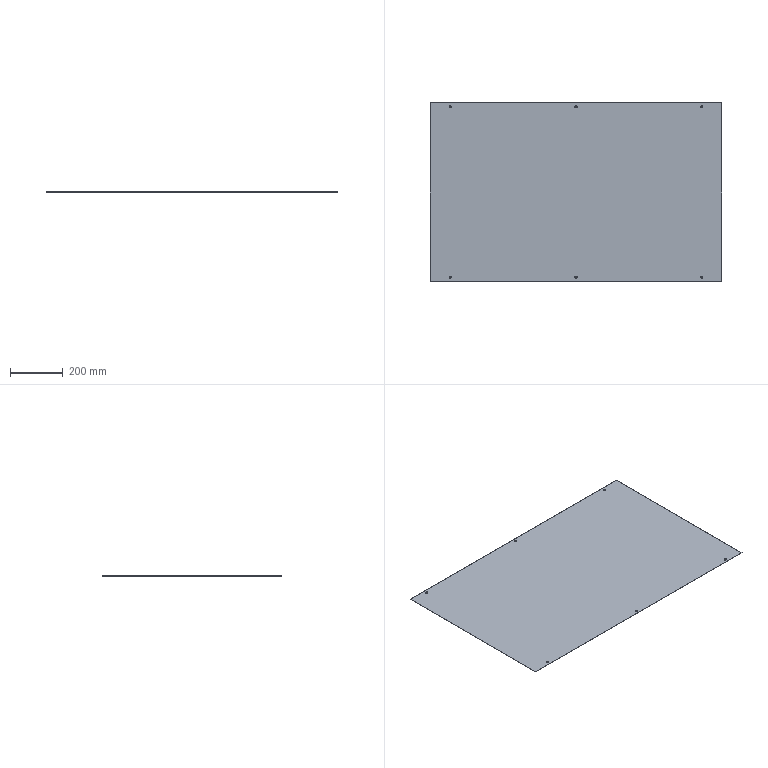Part | SolidWorks | features Cut 1, Extrusion 1 | 1 solid | 18 faces | box 1100 x 672 x 0.8 mm | volume 591119 mm3 | cylinder 12 | plane 6 | commonest cylinder face diameters 8 x12
STEP:
#1=CARTESIAN_POINT('',(-471.,321.,0.8));
#2=VERTEX_POINT('',#1);
#3=CARTESIAN_POINT('',(-479.,321.,0.8));
#4=VERTEX_POINT('',#3);
#5=CARTESIAN_POINT('',(-475.,321.,0.8));
#6=DIRECTION('',(0.,0.,-1.));
#7=DIRECTION('',(-1.,0.,0.));
#8=AXIS2_PLACEMENT_3D('',#5,#6,#7);
#9=CIRCLE('',#8,4.);
#10=EDGE_CURVE('',#2,#4,#9,.T.);
#11=ORIENTED_EDGE('',*,*,#10,.F.);
#12=CARTESIAN_POINT('',(-471.,321.,0.));
#13=VERTEX_POINT('',#12);
#14=CARTESIAN_POINT('',(-471.,321.,0.8));
#15=DIRECTION('',(0.,0.,-1.));
#16=VECTOR('',#15,1000.);
#17=LINE('',#14,#16);
#18=EDGE_CURVE('',#2,#13,#17,.T.);
#19=ORIENTED_EDGE('',*,*,#18,.T.);
#20=CARTESIAN_POINT('',(-479.,321.,0.));
#21=VERTEX_POINT('',#20);
#22=CARTESIAN_POINT('',(-475.,321.,0.));
#23=DIRECTION('',(0.,0.,-1.));
#24=DIRECTION('',(-1.,0.,0.));
#25=AXIS2_PLACEMENT_3D('',#22,#23,#24);
#26=CIRCLE('',#25,4.);
#27=EDGE_CURVE('',#13,#21,#26,.T.);
#28=ORIENTED_EDGE('',*,*,#27,.T.);
#29=CARTESIAN_POINT('',(-479.,321.,0.8));
#30=DIRECTION('',(0.,0.,-1.));
#31=VECTOR('',#30,1000.);
#32=LINE('',#29,#31);
#33=EDGE_CURVE('',#4,#21,#32,.T.);
#34=ORIENTED_EDGE('',*,*,#33,.F.);
#35=EDGE_LOOP('',(#11,#19,#28,#34));
#36=FACE_OUTER_BOUND('',#35,.T.);
#37=CARTESIAN_POINT('',(-475.,321.,0.8));
#38=DIRECTION('',(0.,0.,-1.));
#39=DIRECTION('',(-1.,0.,0.));
#40=AXIS2_PLACEMENT_3D('',#37,#38,#39);
#41=CYLINDRICAL_SURFACE('',#40,4.);
#42=ADVANCED_FACE('',(#36),#41,.F.);
#43=CARTESIAN_POINT('',(479.,321.,0.8));
#44=VERTEX_POINT('',#43);
#45=CARTESIAN_POINT('',(471.,321.,0.8));
#46=VERTEX_POINT('',#45);
#47=CARTESIAN_POINT('',(475.,321.,0.8));
#48=DIRECTION('',(0.,0.,-1.));
#49=DIRECTION('',(1.,0.,0.));
#50=AXIS2_PLACEMENT_3D('',#47,#48,#49);
#51=CIRCLE('',#50,4.);
#52=EDGE_CURVE('',#44,#46,#51,.T.);
#53=ORIENTED_EDGE('',*,*,#52,.F.);
#54=CARTESIAN_POINT('',(479.,321.,0.));
#55=VERTEX_POINT('',#54);
#56=CARTESIAN_POINT('',(479.,321.,0.8));
#57=DIRECTION('',(0.,0.,-1.));
#58=VECTOR('',#57,1000.);
#59=LINE('',#56,#58);
#60=EDGE_CURVE('',#44,#55,#59,.T.);
#61=ORIENTED_EDGE('',*,*,#60,.T.);
#62=CARTESIAN_POINT('',(471.,321.,0.));
#63=VERTEX_POINT('',#62);
#64=CARTESIAN_POINT('',(475.,321.,0.));
#65=DIRECTION('',(0.,0.,-1.));
#66=DIRECTION('',(1.,0.,0.));
#67=AXIS2_PLACEMENT_3D('',#64,#65,#66);
#68=CIRCLE('',#67,4.);
#69=EDGE_CURVE('',#55,#63,#68,.T.);
#70=ORIENTED_EDGE('',*,*,#69,.T.);
#71=CARTESIAN_POINT('',(471.,321.,0.8));
#72=DIRECTION('',(0.,0.,-1.));
#73=VECTOR('',#72,1000.);
#74=LINE('',#71,#73);
#75=EDGE_CURVE('',#46,#63,#74,.T.);
#76=ORIENTED_EDGE('',*,*,#75,.F.);
#77=EDGE_LOOP('',(#53,#61,#70,#76));
#78=FACE_OUTER_BOUND('',#77,.T.);
#79=CARTESIAN_POINT('',(475.,321.,0.8));
#80=DIRECTION('',(0.,0.,-1.));
#81=DIRECTION('',(-1.,0.,0.));
#82=AXIS2_PLACEMENT_3D('',#79,#80,#81);
#83=CYLINDRICAL_SURFACE('',#82,4.);
#84=ADVANCED_FACE('',(#78),#83,.F.);
#85=CARTESIAN_POINT('',(479.,-321.,0.8));
#86=VERTEX_POINT('',#85);
#87=CARTESIAN_POINT('',(471.,-321.,0.8));
#88=VERTEX_POINT('',#87);
#89=CARTESIAN_POINT('',(475.,-321.,0.8));
#90=DIRECTION('',(0.,0.,-1.));
#91=DIRECTION('',(-1.,0.,0.));
#92=AXIS2_PLACEMENT_3D('',#89,#90,#91);
#93=CIRCLE('',#92,4.);
#94=EDGE_CURVE('',#86,#88,#93,.T.);
#95=ORIENTED_EDGE('',*,*,#94,.F.);
#96=CARTESIAN_POINT('',(479.,-321.,0.));
#97=VERTEX_POINT('',#96);
#98=CARTESIAN_POINT('',(479.,-321.,0.8));
#99=DIRECTION('',(0.,0.,-1.));
#100=VECTOR('',#99,1000.);
#101=LINE('',#98,#100);
#102=EDGE_CURVE('',#86,#97,#101,.T.);
#103=ORIENTED_EDGE('',*,*,#102,.T.);
#104=CARTESIAN_POINT('',(471.,-321.,0.));
#105=VERTEX_POINT('',#104);
#106=CARTESIAN_POINT('',(475.,-321.,0.));
#107=DIRECTION('',(0.,0.,-1.));
#108=DIRECTION('',(-1.,0.,0.));
#109=AXIS2_PLACEMENT_3D('',#106,#107,#108);
#110=CIRCLE('',#109,4.);
#111=EDGE_CURVE('',#97,#105,#110,.T.);
#112=ORIENTED_EDGE('',*,*,#111,.T.);
#113=CARTESIAN_POINT('',(471.,-321.,0.8));
#114=DIRECTION('',(0.,0.,-1.));
#115=VECTOR('',#114,1000.);
#116=LINE('',#113,#115);
#117=EDGE_CURVE('',#88,#105,#116,.T.);
#118=ORIENTED_EDGE('',*,*,#117,.F.);
#119=EDGE_LOOP('',(#95,#103,#112,#118));
#120=FACE_OUTER_BOUND('',#119,.T.);
#121=CARTESIAN_POINT('',(475.,-321.,0.8));
#122=DIRECTION('',(0.,0.,-1.));
#123=DIRECTION('',(-1.,0.,0.));
#124=AXIS2_PLACEMENT_3D('',#121,#122,#123);
#125=CYLINDRICAL_SURFACE('',#124,4.);
#126=ADVANCED_FACE('',(#120),#125,.F.);
#127=CARTESIAN_POINT('',(-471.,-321.,0.8));
#128=VERTEX_POINT('',#127);
#129=CARTESIAN_POINT('',(-479.,-321.,0.8));
#130=VERTEX_POINT('',#129);
#131=CARTESIAN_POINT('',(-475.,-321.,0.8));
#132=DIRECTION('',(0.,0.,-1.));
#133=DIRECTION('',(1.,0.,0.));
#134=AXIS2_PLACEMENT_3D('',#131,#132,#133);
#135=CIRCLE('',#134,4.);
#136=EDGE_CURVE('',#128,#130,#135,.T.);
#137=ORIENTED_EDGE('',*,*,#136,.F.);
#138=CARTESIAN_POINT('',(-471.,-321.,0.));
#139=VERTEX_POINT('',#138);
#140=CARTESIAN_POINT('',(-471.,-321.,0.8));
#141=DIRECTION('',(0.,0.,-1.));
#142=VECTOR('',#141,1000.);
#143=LINE('',#140,#142);
#144=EDGE_CURVE('',#128,#139,#143,.T.);
#145=ORIENTED_EDGE('',*,*,#144,.T.);
#146=CARTESIAN_POINT('',(-479.,-321.,0.));
#147=VERTEX_POINT('',#146);
#148=CARTESIAN_POINT('',(-475.,-321.,0.));
#149=DIRECTION('',(0.,0.,-1.));
#150=DIRECTION('',(1.,0.,0.));
#151=AXIS2_PLACEMENT_3D('',#148,#149,#150);
#152=CIRCLE('',#151,4.);
#153=EDGE_CURVE('',#139,#147,#152,.T.);
#154=ORIENTED_EDGE('',*,*,#153,.T.);
#155=CARTESIAN_POINT('',(-479.,-321.,0.8));
#156=DIRECTION('',(0.,0.,-1.));
#157=VECTOR('',#156,1000.);
#158=LINE('',#155,#157);
#159=EDGE_CURVE('',#130,#147,#158,.T.);
#160=ORIENTED_EDGE('',*,*,#159,.F.);
#161=EDGE_LOOP('',(#137,#145,#154,#160));
#162=FACE_OUTER_BOUND('',#161,.T.);
#163=CARTESIAN_POINT('',(-475.,-321.,0.8));
#164=DIRECTION('',(0.,0.,-1.));
#165=DIRECTION('',(-1.,0.,0.));
#166=AXIS2_PLACEMENT_3D('',#163,#164,#165);
#167=CYLINDRICAL_SURFACE('',#166,4.);
#168=ADVANCED_FACE('',(#162),#167,.F.);
#169=CARTESIAN_POINT('',(4.,-321.,0.8));
#170=VERTEX_POINT('',#169);
#171=CARTESIAN_POINT('',(-4.,-321.,0.8));
#172=VERTEX_POINT('',#171);
#173=CARTESIAN_POINT('',(0.,-321.,0.8));
#174=DIRECTION('',(0.,0.,-1.));
#175=DIRECTION('',(1.,0.,0.));
#176=AXIS2_PLACEMENT_3D('',#173,#174,#175);
#177=CIRCLE('',#176,4.);
#178=EDGE_CURVE('',#170,#172,#177,.T.);
#179=ORIENTED_EDGE('',*,*,#178,.F.);
#180=CARTESIAN_POINT('',(4.,-321.,0.));
#181=VERTEX_POINT('',#180);
#182=CARTESIAN_POINT('',(4.,-321.,0.8));
#183=DIRECTION('',(0.,0.,-1.));
#184=VECTOR('',#183,1000.);
#185=LINE('',#182,#184);
#186=EDGE_CURVE('',#170,#181,#185,.T.);
#187=ORIENTED_EDGE('',*,*,#186,.T.);
#188=CARTESIAN_POINT('',(-4.,-321.,0.));
#189=VERTEX_POINT('',#188);
#190=CARTESIAN_POINT('',(0.,-321.,0.));
#191=DIRECTION('',(0.,0.,-1.));
#192=DIRECTION('',(1.,0.,0.));
#193=AXIS2_PLACEMENT_3D('',#190,#191,#192);
#194=CIRCLE('',#193,4.);
#195=EDGE_CURVE('',#181,#189,#194,.T.);
#196=ORIENTED_EDGE('',*,*,#195,.T.);
#197=CARTESIAN_POINT('',(-4.,-321.,0.8));
#198=DIRECTION('',(0.,0.,-1.));
#199=VECTOR('',#198,1000.);
#200=LINE('',#197,#199);
#201=EDGE_CURVE('',#172,#189,#200,.T.);
#202=ORIENTED_EDGE('',*,*,#201,.F.);
#203=EDGE_LOOP('',(#179,#187,#196,#202));
#204=FACE_OUTER_BOUND('',#203,.T.);
#205=CARTESIAN_POINT('',(0.,-321.,0.8));
#206=DIRECTION('',(0.,0.,-1.));
#207=DIRECTION('',(-1.,0.,0.));
#208=AXIS2_PLACEMENT_3D('',#205,#206,#207);
#209=CYLINDRICAL_SURFACE('',#208,4.);
#210=ADVANCED_FACE('',(#204),#209,.F.);
#211=CARTESIAN_POINT('',(4.,321.,0.8));
#212=VERTEX_POINT('',#211);
#213=CARTESIAN_POINT('',(-4.,321.,0.8));
#214=VERTEX_POINT('',#213);
#215=CARTESIAN_POINT('',(0.,321.,0.8));
#216=DIRECTION('',(0.,0.,-1.));
#217=DIRECTION('',(-1.,0.,0.));
#218=AXIS2_PLACEMENT_3D('',#215,#216,#217);
#219=CIRCLE('',#218,4.);
#220=EDGE_CURVE('',#212,#214,#219,.T.);
#221=ORIENTED_EDGE('',*,*,#220,.F.);
#222=CARTESIAN_POINT('',(4.,321.,0.));
#223=VERTEX_POINT('',#222);
#224=CARTESIAN_POINT('',(4.,321.,0.8));
#225=DIRECTION('',(0.,0.,-1.));
#226=VECTOR('',#225,1000.);
#227=LINE('',#224,#226);
#228=EDGE_CURVE('',#212,#223,#227,.T.);
#229=ORIENTED_EDGE('',*,*,#228,.T.);
#230=CARTESIAN_POINT('',(-4.,321.,0.));
#231=VERTEX_POINT('',#230);
#232=CARTESIAN_POINT('',(0.,321.,0.));
#233=DIRECTION('',(0.,0.,-1.));
#234=DIRECTION('',(-1.,0.,0.));
#235=AXIS2_PLACEMENT_3D('',#232,#233,#234);
#236=CIRCLE('',#235,4.);
#237=EDGE_CURVE('',#223,#231,#236,.T.);
#238=ORIENTED_EDGE('',*,*,#237,.T.);
#239=CARTESIAN_POINT('',(-4.,321.,0.8));
#240=DIRECTION('',(0.,0.,-1.));
#241=VECTOR('',#240,1000.);
#242=LINE('',#239,#241);
#243=EDGE_CURVE('',#214,#231,#242,.T.);
#244=ORIENTED_EDGE('',*,*,#243,.F.);
#245=EDGE_LOOP('',(#221,#229,#238,#244));
#246=FACE_OUTER_BOUND('',#245,.T.);
#247=CARTESIAN_POINT('',(0.,321.,0.8));
#248=DIRECTION('',(0.,0.,-1.));
#249=DIRECTION('',(-1.,0.,0.));
#250=AXIS2_PLACEMENT_3D('',#247,#248,#249);
#251=CYLINDRICAL_SURFACE('',#250,4.);
#252=ADVANCED_FACE('',(#246),#251,.F.);
#253=CARTESIAN_POINT('',(550.,-336.,0.));
#254=VERTEX_POINT('',#253);
#255=CARTESIAN_POINT('',(550.,336.,0.));
#256=VERTEX_POINT('',#255);
#257=CARTESIAN_POINT('',(550.,336.,0.));
#258=DIRECTION('',(0.,1.,0.));
#259=VECTOR('',#258,1000.);
#260=LINE('',#257,#259);
#261=EDGE_CURVE('',#254,#256,#260,.T.);
#262=ORIENTED_EDGE('',*,*,#261,.T.);
#263=CARTESIAN_POINT('',(550.,336.,0.8));
#264=VERTEX_POINT('',#263);
#265=CARTESIAN_POINT('',(550.,336.,0.8));
#266=DIRECTION('',(0.,0.,-1.));
#267=VECTOR('',#266,1000.);
#268=LINE('',#265,#267);
#269=EDGE_CURVE('',#264,#256,#268,.T.);
#270=ORIENTED_EDGE('',*,*,#269,.F.);
#271=CARTESIAN_POINT('',(550.,-336.,0.8));
#272=VERTEX_POINT('',#271);
#273=CARTESIAN_POINT('',(550.,336.,0.8));
#274=DIRECTION('',(0.,1.,0.));
#275=VECTOR('',#274,1000.);
#276=LINE('',#273,#275);
#277=EDGE_CURVE('',#272,#264,#276,.T.);
#278=ORIENTED_EDGE('',*,*,#277,.F.);
#279=CARTESIAN_POINT('',(550.,-336.,0.8));
#280=DIRECTION('',(0.,0.,-1.));
#281=VECTOR('',#280,1000.);
#282=LINE('',#279,#281);
#283=EDGE_CURVE('',#272,#254,#282,.T.);
#284=ORIENTED_EDGE('',*,*,#283,.T.);
#285=EDGE_LOOP('',(#262,#270,#278,#284));
#286=FACE_OUTER_BOUND('',#285,.T.);
#287=CARTESIAN_POINT('',(550.,336.,0.8));
#288=DIRECTION('',(-1.,0.,0.));
#289=DIRECTION('',(0.,-1.,0.));
#290=AXIS2_PLACEMENT_3D('',#287,#288,#289);
#291=PLANE('',#290);
#292=ADVANCED_FACE('',(#286),#291,.F.);
#293=CARTESIAN_POINT('',(-550.,336.,0.));
#294=VERTEX_POINT('',#293);
#295=CARTESIAN_POINT('',(-550.,336.,0.));
#296=DIRECTION('',(-1.,0.,0.));
#297=VECTOR('',#296,1000.);
#298=LINE('',#295,#297);
#299=EDGE_CURVE('',#256,#294,#298,.T.);
#300=ORIENTED_EDGE('',*,*,#299,.T.);
#301=CARTESIAN_POINT('',(-550.,336.,0.8));
#302=VERTEX_POINT('',#301);
#303=CARTESIAN_POINT('',(-550.,336.,0.8));
#304=DIRECTION('',(0.,0.,-1.));
#305=VECTOR('',#304,1000.);
#306=LINE('',#303,#305);
#307=EDGE_CURVE('',#302,#294,#306,.T.);
#308=ORIENTED_EDGE('',*,*,#307,.F.);
#309=CARTESIAN_POINT('',(-550.,336.,0.8));
#310=DIRECTION('',(-1.,0.,0.));
#311=VECTOR('',#310,1000.);
#312=LINE('',#309,#311);
#313=EDGE_CURVE('',#264,#302,#312,.T.);
#314=ORIENTED_EDGE('',*,*,#313,.F.);
#315=ORIENTED_EDGE('',*,*,#269,.T.);
#316=EDGE_LOOP('',(#300,#308,#314,#315));
#317=FACE_OUTER_BOUND('',#316,.T.);
#318=CARTESIAN_POINT('',(-550.,336.,0.8));
#319=DIRECTION('',(0.,-1.,0.));
#320=DIRECTION('',(0.,0.,-1.));
#321=AXIS2_PLACEMENT_3D('',#318,#319,#320);
#322=PLANE('',#321);
#323=ADVANCED_FACE('',(#317),#322,.F.);
#324=CARTESIAN_POINT('',(-550.,-336.,0.));
#325=VERTEX_POINT('',#324);
#326=CARTESIAN_POINT('',(-550.,336.,0.));
#327=DIRECTION('',(0.,-1.,0.));
#328=VECTOR('',#327,1000.);
#329=LINE('',#326,#328);
#330=EDGE_CURVE('',#294,#325,#329,.T.);
#331=ORIENTED_EDGE('',*,*,#330,.T.);
#332=CARTESIAN_POINT('',(-550.,-336.,0.8));
#333=VERTEX_POINT('',#332);
#334=CARTESIAN_POINT('',(-550.,-336.,0.8));
#335=DIRECTION('',(0.,0.,-1.));
#336=VECTOR('',#335,1000.);
#337=LINE('',#334,#336);
#338=EDGE_CURVE('',#333,#325,#337,.T.);
#339=ORIENTED_EDGE('',*,*,#338,.F.);
#340=CARTESIAN_POINT('',(-550.,336.,0.8));
#341=DIRECTION('',(0.,-1.,0.));
#342=VECTOR('',#341,1000.);
#343=LINE('',#340,#342);
#344=EDGE_CURVE('',#302,#333,#343,.T.);
#345=ORIENTED_EDGE('',*,*,#344,.F.);
#346=ORIENTED_EDGE('',*,*,#307,.T.);
#347=EDGE_LOOP('',(#331,#339,#345,#346));
#348=FACE_OUTER_BOUND('',#347,.T.);
#349=CARTESIAN_POINT('',(-550.,336.,0.8));
#350=DIRECTION('',(1.,0.,0.));
#351=DIRECTION('',(0.,1.,0.));
#352=AXIS2_PLACEMENT_3D('',#349,#350,#351);
#353=PLANE('',#352);
#354=ADVANCED_FACE('',(#348),#353,.F.);
#355=CARTESIAN_POINT('',(-550.,-336.,0.));
#356=DIRECTION('',(1.,0.,0.));
#357=VECTOR('',#356,1000.);
#358=LINE('',#355,#357);
#359=EDGE_CURVE('',#325,#254,#358,.T.);
#360=ORIENTED_EDGE('',*,*,#359,.T.);
#361=ORIENTED_EDGE('',*,*,#283,.F.);
#362=CARTESIAN_POINT('',(-550.,-336.,0.8));
#363=DIRECTION('',(1.,0.,0.));
#364=VECTOR('',#363,1000.);
#365=LINE('',#362,#364);
#366=EDGE_CURVE('',#333,#272,#365,.T.);
#367=ORIENTED_EDGE('',*,*,#366,.F.);
#368=ORIENTED_EDGE('',*,*,#338,.T.);
#369=EDGE_LOOP('',(#360,#361,#367,#368));
#370=FACE_OUTER_BOUND('',#369,.T.);
#371=CARTESIAN_POINT('',(-550.,-336.,0.8));
#372=DIRECTION('',(0.,1.,0.));
#373=DIRECTION('',(0.,0.,1.));
#374=AXIS2_PLACEMENT_3D('',#371,#372,#373);
#375=PLANE('',#374);
#376=ADVANCED_FACE('',(#370),#375,.F.);
#377=CARTESIAN_POINT('',(-475.,321.,0.8));
#378=DIRECTION('',(0.,0.,-1.));
#379=DIRECTION('',(-1.,0.,0.));
#380=AXIS2_PLACEMENT_3D('',#377,#378,#379);
#381=CIRCLE('',#380,4.);
#382=EDGE_CURVE('',#4,#2,#381,.T.);
#383=ORIENTED_EDGE('',*,*,#382,.T.);
#384=ORIENTED_EDGE('',*,*,#10,.T.);
#385=EDGE_LOOP('',(#383,#384));
#386=FACE_BOUND('',#385,.T.);
#387=CARTESIAN_POINT('',(475.,321.,0.8));
#388=DIRECTION('',(0.,0.,-1.));
#389=DIRECTION('',(1.,0.,0.));
#390=AXIS2_PLACEMENT_3D('',#387,#388,#389);
#391=CIRCLE('',#390,4.);
#392=EDGE_CURVE('',#46,#44,#391,.T.);
#393=ORIENTED_EDGE('',*,*,#392,.T.);
#394=ORIENTED_EDGE('',*,*,#52,.T.);
#395=EDGE_LOOP('',(#393,#394));
#396=FACE_BOUND('',#395,.T.);
#397=CARTESIAN_POINT('',(475.,-321.,0.8));
#398=DIRECTION('',(0.,0.,-1.));
#399=DIRECTION('',(-1.,0.,0.));
#400=AXIS2_PLACEMENT_3D('',#397,#398,#399);
#401=CIRCLE('',#400,4.);
#402=EDGE_CURVE('',#88,#86,#401,.T.);
#403=ORIENTED_EDGE('',*,*,#402,.T.);
#404=ORIENTED_EDGE('',*,*,#94,.T.);
#405=EDGE_LOOP('',(#403,#404));
#406=FACE_BOUND('',#405,.T.);
#407=CARTESIAN_POINT('',(-475.,-321.,0.8));
#408=DIRECTION('',(0.,0.,-1.));
#409=DIRECTION('',(1.,0.,0.));
#410=AXIS2_PLACEMENT_3D('',#407,#408,#409);
#411=CIRCLE('',#410,4.);
#412=EDGE_CURVE('',#130,#128,#411,.T.);
#413=ORIENTED_EDGE('',*,*,#412,.T.);
#414=ORIENTED_EDGE('',*,*,#136,.T.);
#415=EDGE_LOOP('',(#413,#414));
#416=FACE_BOUND('',#415,.T.);
#417=CARTESIAN_POINT('',(0.,-321.,0.8));
#418=DIRECTION('',(0.,0.,-1.));
#419=DIRECTION('',(1.,0.,0.));
#420=AXIS2_PLACEMENT_3D('',#417,#418,#419);
#421=CIRCLE('',#420,4.);
#422=EDGE_CURVE('',#172,#170,#421,.T.);
#423=ORIENTED_EDGE('',*,*,#422,.T.);
#424=ORIENTED_EDGE('',*,*,#178,.T.);
#425=EDGE_LOOP('',(#423,#424));
#426=FACE_BOUND('',#425,.T.);
#427=CARTESIAN_POINT('',(0.,321.,0.8));
#428=DIRECTION('',(0.,0.,-1.));
#429=DIRECTION('',(-1.,0.,0.));
#430=AXIS2_PLACEMENT_3D('',#427,#428,#429);
#431=CIRCLE('',#430,4.);
#432=EDGE_CURVE('',#214,#212,#431,.T.);
#433=ORIENTED_EDGE('',*,*,#432,.T.);
#434=ORIENTED_EDGE('',*,*,#220,.T.);
#435=EDGE_LOOP('',(#433,#434));
#436=FACE_BOUND('',#435,.T.);
#437=ORIENTED_EDGE('',*,*,#277,.T.);
#438=ORIENTED_EDGE('',*,*,#313,.T.);
#439=ORIENTED_EDGE('',*,*,#344,.T.);
#440=ORIENTED_EDGE('',*,*,#366,.T.);
#441=EDGE_LOOP('',(#437,#438,#439,#440));
#442=FACE_OUTER_BOUND('',#441,.T.);
#443=CARTESIAN_POINT('',(0.,0.,0.8));
#444=DIRECTION('',(0.,0.,1.));
#445=DIRECTION('',(1.,0.,0.));
#446=AXIS2_PLACEMENT_3D('',#443,#444,#445);
#447=PLANE('',#446);
#448=ADVANCED_FACE('',(#386,#396,#406,#416,#426,#436,#442),#447,.T.);
#449=CARTESIAN_POINT('',(-475.,321.,0.));
#450=DIRECTION('',(0.,0.,-1.));
#451=DIRECTION('',(-1.,0.,0.));
#452=AXIS2_PLACEMENT_3D('',#449,#450,#451);
#453=CIRCLE('',#452,4.);
#454=EDGE_CURVE('',#21,#13,#453,.T.);
#455=ORIENTED_EDGE('',*,*,#454,.F.);
#456=ORIENTED_EDGE('',*,*,#27,.F.);
#457=EDGE_LOOP('',(#455,#456));
#458=FACE_BOUND('',#457,.T.);
#459=CARTESIAN_POINT('',(475.,321.,0.));
#460=DIRECTION('',(0.,0.,-1.));
#461=DIRECTION('',(1.,0.,0.));
#462=AXIS2_PLACEMENT_3D('',#459,#460,#461);
#463=CIRCLE('',#462,4.);
#464=EDGE_CURVE('',#63,#55,#463,.T.);
#465=ORIENTED_EDGE('',*,*,#464,.F.);
#466=ORIENTED_EDGE('',*,*,#69,.F.);
#467=EDGE_LOOP('',(#465,#466));
#468=FACE_BOUND('',#467,.T.);
#469=CARTESIAN_POINT('',(475.,-321.,0.));
#470=DIRECTION('',(0.,0.,-1.));
#471=DIRECTION('',(-1.,0.,0.));
#472=AXIS2_PLACEMENT_3D('',#469,#470,#471);
#473=CIRCLE('',#472,4.);
#474=EDGE_CURVE('',#105,#97,#473,.T.);
#475=ORIENTED_EDGE('',*,*,#474,.F.);
#476=ORIENTED_EDGE('',*,*,#111,.F.);
#477=EDGE_LOOP('',(#475,#476));
#478=FACE_BOUND('',#477,.T.);
#479=CARTESIAN_POINT('',(-475.,-321.,0.));
#480=DIRECTION('',(0.,0.,-1.));
#481=DIRECTION('',(1.,0.,0.));
#482=AXIS2_PLACEMENT_3D('',#479,#480,#481);
#483=CIRCLE('',#482,4.);
#484=EDGE_CURVE('',#147,#139,#483,.T.);
#485=ORIENTED_EDGE('',*,*,#484,.F.);
#486=ORIENTED_EDGE('',*,*,#153,.F.);
#487=EDGE_LOOP('',(#485,#486));
#488=FACE_BOUND('',#487,.T.);
#489=CARTESIAN_POINT('',(0.,-321.,0.));
#490=DIRECTION('',(0.,0.,-1.));
#491=DIRECTION('',(1.,0.,0.));
#492=AXIS2_PLACEMENT_3D('',#489,#490,#491);
#493=CIRCLE('',#492,4.);
#494=EDGE_CURVE('',#189,#181,#493,.T.);
#495=ORIENTED_EDGE('',*,*,#494,.F.);
#496=ORIENTED_EDGE('',*,*,#195,.F.);
#497=EDGE_LOOP('',(#495,#496));
#498=FACE_BOUND('',#497,.T.);
#499=CARTESIAN_POINT('',(0.,321.,0.));
#500=DIRECTION('',(0.,0.,-1.));
#501=DIRECTION('',(-1.,0.,0.));
#502=AXIS2_PLACEMENT_3D('',#499,#500,#501);
#503=CIRCLE('',#502,4.);
#504=EDGE_CURVE('',#231,#223,#503,.T.);
#505=ORIENTED_EDGE('',*,*,#504,.F.);
#506=ORIENTED_EDGE('',*,*,#237,.F.);
#507=EDGE_LOOP('',(#505,#506));
#508=FACE_BOUND('',#507,.T.);
#509=ORIENTED_EDGE('',*,*,#261,.F.);
#510=ORIENTED_EDGE('',*,*,#359,.F.);
#511=ORIENTED_EDGE('',*,*,#330,.F.);
#512=ORIENTED_EDGE('',*,*,#299,.F.);
#513=EDGE_LOOP('',(#509,#510,#511,#512));
#514=FACE_OUTER_BOUND('',#513,.T.);
#515=CARTESIAN_POINT('',(0.,0.,0.));
#516=DIRECTION('',(0.,0.,1.));
#517=DIRECTION('',(1.,0.,0.));
#518=AXIS2_PLACEMENT_3D('',#515,#516,#517);
#519=PLANE('',#518);
#520=ADVANCED_FACE('',(#458,#468,#478,#488,#498,#508,#514),#519,.F.);
#521=ORIENTED_EDGE('',*,*,#228,.F.);
#522=ORIENTED_EDGE('',*,*,#432,.F.);
#523=ORIENTED_EDGE('',*,*,#243,.T.);
#524=ORIENTED_EDGE('',*,*,#504,.T.);
#525=EDGE_LOOP('',(#521,#522,#523,#524));
#526=FACE_OUTER_BOUND('',#525,.T.);
#527=CARTESIAN_POINT('',(0.,321.,0.8));
#528=DIRECTION('',(0.,0.,-1.));
#529=DIRECTION('',(-1.,0.,0.));
#530=AXIS2_PLACEMENT_3D('',#527,#528,#529);
#531=CYLINDRICAL_SURFACE('',#530,4.);
#532=ADVANCED_FACE('',(#526),#531,.F.);
#533=ORIENTED_EDGE('',*,*,#186,.F.);
#534=ORIENTED_EDGE('',*,*,#422,.F.);
#535=ORIENTED_EDGE('',*,*,#201,.T.);
#536=ORIENTED_EDGE('',*,*,#494,.T.);
#537=EDGE_LOOP('',(#533,#534,#535,#536));
#538=FACE_OUTER_BOUND('',#537,.T.);
#539=CARTESIAN_POINT('',(0.,-321.,0.8));
#540=DIRECTION('',(0.,0.,-1.));
#541=DIRECTION('',(-1.,0.,0.));
#542=AXIS2_PLACEMENT_3D('',#539,#540,#541);
#543=CYLINDRICAL_SURFACE('',#542,4.);
#544=ADVANCED_FACE('',(#538),#543,.F.);
#545=ORIENTED_EDGE('',*,*,#144,.F.);
#546=ORIENTED_EDGE('',*,*,#412,.F.);
#547=ORIENTED_EDGE('',*,*,#159,.T.);
#548=ORIENTED_EDGE('',*,*,#484,.T.);
#549=EDGE_LOOP('',(#545,#546,#547,#548));
#550=FACE_OUTER_BOUND('',#549,.T.);
#551=CARTESIAN_POINT('',(-475.,-321.,0.8));
#552=DIRECTION('',(0.,0.,-1.));
#553=DIRECTION('',(-1.,0.,0.));
#554=AXIS2_PLACEMENT_3D('',#551,#552,#553);
#555=CYLINDRICAL_SURFACE('',#554,4.);
#556=ADVANCED_FACE('',(#550),#555,.F.);
#557=ORIENTED_EDGE('',*,*,#102,.F.);
#558=ORIENTED_EDGE('',*,*,#402,.F.);
#559=ORIENTED_EDGE('',*,*,#117,.T.);
#560=ORIENTED_EDGE('',*,*,#474,.T.);
#561=EDGE_LOOP('',(#557,#558,#559,#560));
#562=FACE_OUTER_BOUND('',#561,.T.);
#563=CARTESIAN_POINT('',(475.,-321.,0.8));
#564=DIRECTION('',(0.,0.,-1.));
#565=DIRECTION('',(-1.,0.,0.));
#566=AXIS2_PLACEMENT_3D('',#563,#564,#565);
#567=CYLINDRICAL_SURFACE('',#566,4.);
#568=ADVANCED_FACE('',(#562),#567,.F.);
#569=ORIENTED_EDGE('',*,*,#60,.F.);
#570=ORIENTED_EDGE('',*,*,#392,.F.);
#571=ORIENTED_EDGE('',*,*,#75,.T.);
#572=ORIENTED_EDGE('',*,*,#464,.T.);
#573=EDGE_LOOP('',(#569,#570,#571,#572));
#574=FACE_OUTER_BOUND('',#573,.T.);
#575=CARTESIAN_POINT('',(475.,321.,0.8));
#576=DIRECTION('',(0.,0.,-1.));
#577=DIRECTION('',(-1.,0.,0.));
#578=AXIS2_PLACEMENT_3D('',#575,#576,#577);
#579=CYLINDRICAL_SURFACE('',#578,4.);
#580=ADVANCED_FACE('',(#574),#579,.F.);
#581=ORIENTED_EDGE('',*,*,#18,.F.);
#582=ORIENTED_EDGE('',*,*,#382,.F.);
#583=ORIENTED_EDGE('',*,*,#33,.T.);
#584=ORIENTED_EDGE('',*,*,#454,.T.);
#585=EDGE_LOOP('',(#581,#582,#583,#584));
#586=FACE_OUTER_BOUND('',#585,.T.);
#587=CARTESIAN_POINT('',(-475.,321.,0.8));
#588=DIRECTION('',(0.,0.,-1.));
#589=DIRECTION('',(-1.,0.,0.));
#590=AXIS2_PLACEMENT_3D('',#587,#588,#589);
#591=CYLINDRICAL_SURFACE('',#590,4.);
#592=ADVANCED_FACE('',(#586),#591,.F.);
#593=CLOSED_SHELL('',(#42,#84,#126,#168,#210,#252,#292,#323,#354,#376,#448,#520,#532,#544,#556,#568,#580,#592));
#594=MANIFOLD_SOLID_BREP('',#593);
#595=CARTESIAN_POINT('',(0.,0.,0.));
#596=DIRECTION('',(0.,0.,1.));
#597=DIRECTION('',(1.,0.,0.));
#598=AXIS2_PLACEMENT_3D('',#595,#596,#597);
#599=(LENGTH_UNIT()NAMED_UNIT(*)SI_UNIT(.MILLI.,.METRE.));
#600=UNCERTAINTY_MEASURE_WITH_UNIT(LENGTH_MEASURE(0.00001),#599,'','');
#601=(NAMED_UNIT(*)PLANE_ANGLE_UNIT()SI_UNIT($,.RADIAN.));
#602=(NAMED_UNIT(*)SI_UNIT($,.STERADIAN.)SOLID_ANGLE_UNIT());
#603=(GEOMETRIC_REPRESENTATION_CONTEXT(3)GLOBAL_UNCERTAINTY_ASSIGNED_CONTEXT((#600))GLOBAL_UNIT_ASSIGNED_CONTEXT((#599,#601,#602))REPRESENTATION_CONTEXT('',''));
#604=ADVANCED_BREP_SHAPE_REPRESENTATION('',(#594,#598),#603);